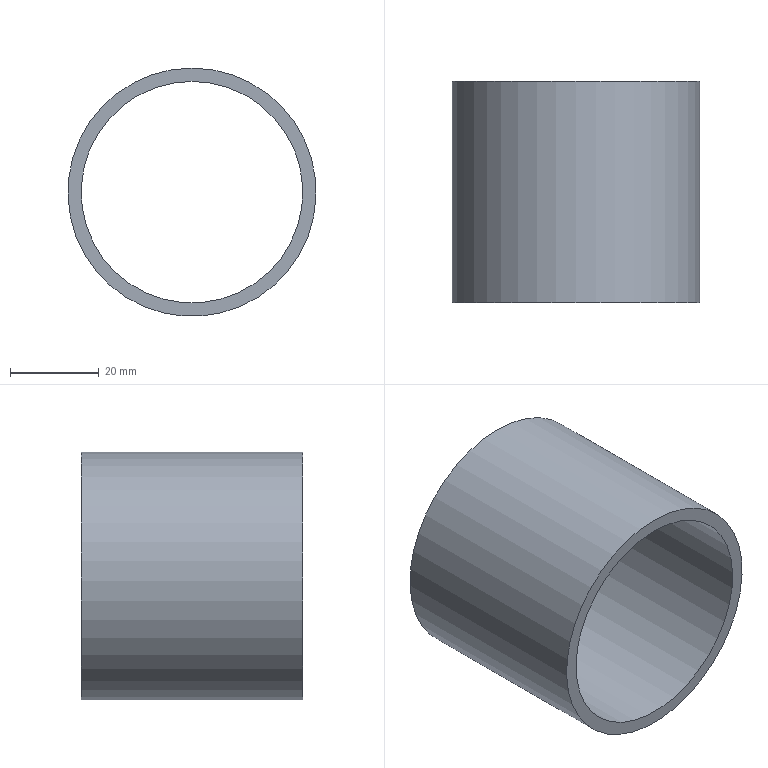Part | STEP file | JBJ-P-1003-08 | 1 solid | 4 faces | box 56 x 50 x 56 mm | volume 24976 mm3 | plane 2 | cylinder 2 | commonest cylinder face diameters 50 x1 56 x1
STEP:
#1=CARTESIAN_POINT('',(0.,50.,28.));
#2=VERTEX_POINT('',#1);
#3=CARTESIAN_POINT('',(0.,50.,0.));
#4=DIRECTION('',(0.,1.,0.));
#5=DIRECTION('',(0.,0.,1.));
#6=AXIS2_PLACEMENT_3D('',#3,#4,#5);
#7=CIRCLE('',#6,28.);
#8=EDGE_CURVE('',#2,#2,#7,.T.);
#9=ORIENTED_EDGE('',*,*,#8,.T.);
#10=EDGE_LOOP('',(#9));
#11=FACE_OUTER_BOUND('',#10,.T.);
#12=CARTESIAN_POINT('',(0.,50.,25.));
#13=VERTEX_POINT('',#12);
#14=CARTESIAN_POINT('',(0.,50.,0.));
#15=DIRECTION('',(0.,1.,0.));
#16=DIRECTION('',(0.,0.,1.));
#17=AXIS2_PLACEMENT_3D('',#14,#15,#16);
#18=CIRCLE('',#17,25.);
#19=EDGE_CURVE('',#13,#13,#18,.T.);
#20=ORIENTED_EDGE('',*,*,#19,.F.);
#21=EDGE_LOOP('',(#20));
#22=FACE_BOUND('',#21,.T.);
#23=CARTESIAN_POINT('',(0.,50.,0.));
#24=DIRECTION('',(0.,1.,0.));
#25=DIRECTION('',(0.,0.,1.));
#26=AXIS2_PLACEMENT_3D('',#23,#24,#25);
#27=PLANE('',#26);
#28=ADVANCED_FACE('',(#11,#22),#27,.T.);
#29=CARTESIAN_POINT('',(0.,0.,28.));
#30=VERTEX_POINT('',#29);
#31=CARTESIAN_POINT('',(0.,0.,0.));
#32=DIRECTION('',(0.,1.,0.));
#33=DIRECTION('',(0.,0.,1.));
#34=AXIS2_PLACEMENT_3D('',#31,#32,#33);
#35=CIRCLE('',#34,28.);
#36=EDGE_CURVE('',#30,#30,#35,.T.);
#37=ORIENTED_EDGE('',*,*,#36,.F.);
#38=EDGE_LOOP('',(#37));
#39=FACE_OUTER_BOUND('',#38,.T.);
#40=CARTESIAN_POINT('',(0.,0.,25.));
#41=VERTEX_POINT('',#40);
#42=CARTESIAN_POINT('',(0.,0.,0.));
#43=DIRECTION('',(0.,1.,0.));
#44=DIRECTION('',(0.,0.,1.));
#45=AXIS2_PLACEMENT_3D('',#42,#43,#44);
#46=CIRCLE('',#45,25.);
#47=EDGE_CURVE('',#41,#41,#46,.T.);
#48=ORIENTED_EDGE('',*,*,#47,.T.);
#49=EDGE_LOOP('',(#48));
#50=FACE_BOUND('',#49,.T.);
#51=CARTESIAN_POINT('',(0.,0.,0.));
#52=DIRECTION('',(0.,1.,0.));
#53=DIRECTION('',(0.,0.,1.));
#54=AXIS2_PLACEMENT_3D('',#51,#52,#53);
#55=PLANE('',#54);
#56=ADVANCED_FACE('',(#39,#50),#55,.F.);
#57=ORIENTED_EDGE('',*,*,#8,.F.);
#58=EDGE_LOOP('',(#57));
#59=FACE_OUTER_BOUND('',#58,.T.);
#60=ORIENTED_EDGE('',*,*,#36,.T.);
#61=EDGE_LOOP('',(#60));
#62=FACE_OUTER_BOUND('',#61,.T.);
#63=CARTESIAN_POINT('',(0.,50.,0.));
#64=DIRECTION('',(0.,-1.,0.));
#65=DIRECTION('',(0.,0.,-1.));
#66=AXIS2_PLACEMENT_3D('',#63,#64,#65);
#67=CYLINDRICAL_SURFACE('',#66,28.);
#68=ADVANCED_FACE('',(#59,#62),#67,.T.);
#69=ORIENTED_EDGE('',*,*,#19,.T.);
#70=EDGE_LOOP('',(#69));
#71=FACE_OUTER_BOUND('',#70,.T.);
#72=ORIENTED_EDGE('',*,*,#47,.F.);
#73=EDGE_LOOP('',(#72));
#74=FACE_OUTER_BOUND('',#73,.T.);
#75=CARTESIAN_POINT('',(0.,50.,0.));
#76=DIRECTION('',(0.,-1.,0.));
#77=DIRECTION('',(0.,0.,-1.));
#78=AXIS2_PLACEMENT_3D('',#75,#76,#77);
#79=CYLINDRICAL_SURFACE('',#78,25.);
#80=ADVANCED_FACE('',(#71,#74),#79,.F.);
#81=CLOSED_SHELL('',(#28,#56,#68,#80));
#82=MANIFOLD_SOLID_BREP('',#81);
#83=CARTESIAN_POINT('',(0.,0.,0.));
#84=DIRECTION('',(0.,0.,1.));
#85=DIRECTION('',(1.,0.,0.));
#86=AXIS2_PLACEMENT_3D('',#83,#84,#85);
#87=(LENGTH_UNIT()NAMED_UNIT(*)SI_UNIT(.MILLI.,.METRE.));
#88=UNCERTAINTY_MEASURE_WITH_UNIT(LENGTH_MEASURE(0.00001),#87,'','');
#89=(NAMED_UNIT(*)PLANE_ANGLE_UNIT()SI_UNIT($,.RADIAN.));
#90=(NAMED_UNIT(*)SI_UNIT($,.STERADIAN.)SOLID_ANGLE_UNIT());
#91=(GEOMETRIC_REPRESENTATION_CONTEXT(3)GLOBAL_UNCERTAINTY_ASSIGNED_CONTEXT((#88))GLOBAL_UNIT_ASSIGNED_CONTEXT((#87,#89,#90))REPRESENTATION_CONTEXT('',''));
#92=ADVANCED_BREP_SHAPE_REPRESENTATION('',(#82,#86),#91);